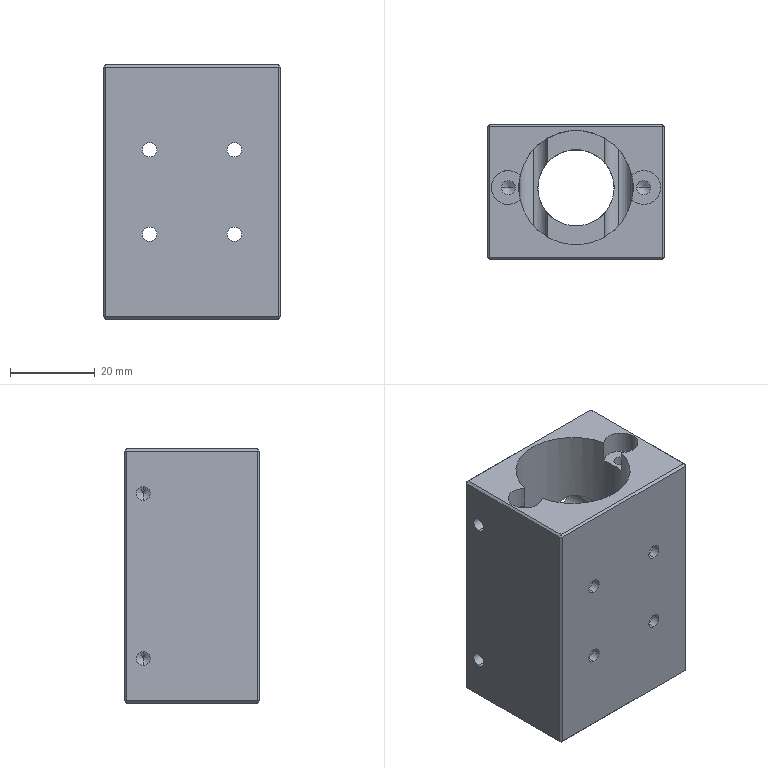Part | SolidWorks | features BaseBody 1 | 1 solid | 103 faces | box 42 x 32 x 60 mm | volume 48942 mm3 | cylinder 47 | plane 36 | cone 20 | commonest cylinder face diameters 3.3 x20 6.5 x12 3.4 x8 8 x3 18 x2 27 x2